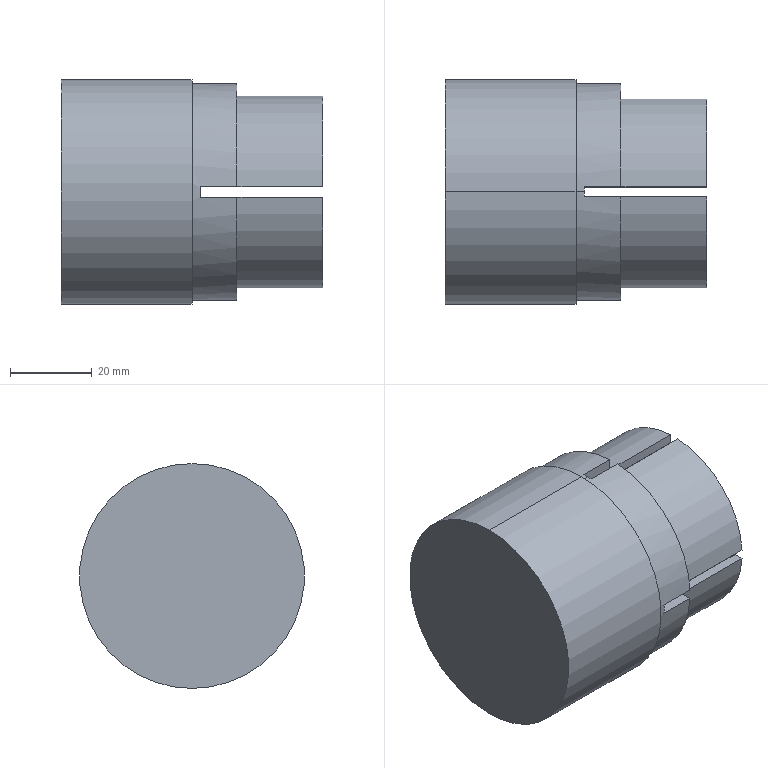Part | SolidWorks | features BaseBody 1 | 1 solid | 37 faces | box 64 x 55 x 55 mm | volume 51212 mm3 | plane 26 | cylinder 11 | commonest cylinder face diameters 47 x4 42.2 x3 53 x2 55 x2
STEP:
#1=CARTESIAN_POINT('',(34.,-1.25,-21.063));
#2=VERTEX_POINT('',#1);
#3=CARTESIAN_POINT('',(34.,0.,-21.1));
#4=VERTEX_POINT('',#3);
#5=CARTESIAN_POINT('',(34.,0.,0.));
#6=DIRECTION('',(1.,0.,0.));
#7=DIRECTION('',(0.,0.,1.));
#8=AXIS2_PLACEMENT_3D('',#5,#6,#7);
#9=CIRCLE('',#8,21.1);
#10=EDGE_CURVE('',#2,#4,#9,.T.);
#11=ORIENTED_EDGE('',*,*,#10,.T.);
#12=CARTESIAN_POINT('',(5.,0.,-21.1));
#13=VERTEX_POINT('',#12);
#14=CARTESIAN_POINT('',(-11.146,0.,-21.1));
#15=DIRECTION('',(-1.,0.,0.));
#16=VECTOR('',#15,1000.);
#17=LINE('',#14,#16);
#18=EDGE_CURVE('',#4,#13,#17,.T.);
#19=ORIENTED_EDGE('',*,*,#18,.T.);
#20=CARTESIAN_POINT('',(5.,0.,21.1));
#21=VERTEX_POINT('',#20);
#22=CARTESIAN_POINT('',(5.,0.,0.));
#23=DIRECTION('',(1.,0.,0.));
#24=DIRECTION('',(0.,0.,1.));
#25=AXIS2_PLACEMENT_3D('',#22,#23,#24);
#26=CIRCLE('',#25,21.1);
#27=EDGE_CURVE('',#21,#13,#26,.T.);
#28=ORIENTED_EDGE('',*,*,#27,.F.);
#29=CARTESIAN_POINT('',(34.,0.,21.1));
#30=VERTEX_POINT('',#29);
#31=CARTESIAN_POINT('',(-11.146,0.,21.1));
#32=DIRECTION('',(-1.,0.,0.));
#33=VECTOR('',#32,1000.);
#34=LINE('',#31,#33);
#35=EDGE_CURVE('',#30,#21,#34,.T.);
#36=ORIENTED_EDGE('',*,*,#35,.F.);
#37=CARTESIAN_POINT('',(34.,-1.25,21.063));
#38=VERTEX_POINT('',#37);
#39=CARTESIAN_POINT('',(34.,0.,0.));
#40=DIRECTION('',(1.,0.,0.));
#41=DIRECTION('',(0.,0.,1.));
#42=AXIS2_PLACEMENT_3D('',#39,#40,#41);
#43=CIRCLE('',#42,21.1);
#44=EDGE_CURVE('',#30,#38,#43,.T.);
#45=ORIENTED_EDGE('',*,*,#44,.T.);
#46=CARTESIAN_POINT('',(64.,-1.25,21.063));
#47=VERTEX_POINT('',#46);
#48=CARTESIAN_POINT('',(-11.146,-1.25,21.063));
#49=DIRECTION('',(-1.,0.,0.));
#50=VECTOR('',#49,1000.);
#51=LINE('',#48,#50);
#52=EDGE_CURVE('',#47,#38,#51,.T.);
#53=ORIENTED_EDGE('',*,*,#52,.F.);
#54=CARTESIAN_POINT('',(64.,-21.063,1.25));
#55=VERTEX_POINT('',#54);
#56=CARTESIAN_POINT('',(64.,0.,0.));
#57=DIRECTION('',(-1.,0.,0.));
#58=DIRECTION('',(0.,0.,1.));
#59=AXIS2_PLACEMENT_3D('',#56,#57,#58);
#60=CIRCLE('',#59,21.1);
#61=EDGE_CURVE('',#55,#47,#60,.T.);
#62=ORIENTED_EDGE('',*,*,#61,.F.);
#63=CARTESIAN_POINT('',(34.,-21.063,1.25));
#64=VERTEX_POINT('',#63);
#65=CARTESIAN_POINT('',(-11.146,-21.063,1.25));
#66=DIRECTION('',(1.,0.,0.));
#67=VECTOR('',#66,1000.);
#68=LINE('',#65,#67);
#69=EDGE_CURVE('',#64,#55,#68,.T.);
#70=ORIENTED_EDGE('',*,*,#69,.F.);
#71=CARTESIAN_POINT('',(34.,-21.063,-1.25));
#72=VERTEX_POINT('',#71);
#73=CARTESIAN_POINT('',(34.,0.,0.));
#74=DIRECTION('',(-1.,0.,0.));
#75=DIRECTION('',(0.,0.,1.));
#76=AXIS2_PLACEMENT_3D('',#73,#74,#75);
#77=CIRCLE('',#76,21.1);
#78=EDGE_CURVE('',#72,#64,#77,.T.);
#79=ORIENTED_EDGE('',*,*,#78,.F.);
#80=CARTESIAN_POINT('',(64.,-21.063,-1.25));
#81=VERTEX_POINT('',#80);
#82=CARTESIAN_POINT('',(-11.146,-21.063,-1.25));
#83=DIRECTION('',(-1.,0.,0.));
#84=VECTOR('',#83,1000.);
#85=LINE('',#82,#84);
#86=EDGE_CURVE('',#81,#72,#85,.T.);
#87=ORIENTED_EDGE('',*,*,#86,.F.);
#88=CARTESIAN_POINT('',(64.,-1.25,-21.063));
#89=VERTEX_POINT('',#88);
#90=CARTESIAN_POINT('',(64.,0.,0.));
#91=DIRECTION('',(-1.,0.,0.));
#92=DIRECTION('',(0.,0.,1.));
#93=AXIS2_PLACEMENT_3D('',#90,#91,#92);
#94=CIRCLE('',#93,21.1);
#95=EDGE_CURVE('',#89,#81,#94,.T.);
#96=ORIENTED_EDGE('',*,*,#95,.F.);
#97=CARTESIAN_POINT('',(-11.146,-1.25,-21.063));
#98=DIRECTION('',(1.,0.,0.));
#99=VECTOR('',#98,1000.);
#100=LINE('',#97,#99);
#101=EDGE_CURVE('',#2,#89,#100,.T.);
#102=ORIENTED_EDGE('',*,*,#101,.F.);
#103=EDGE_LOOP('',(#11,#19,#28,#36,#45,#53,#62,#70,#79,#87,#96,#102));
#104=FACE_OUTER_BOUND('',#103,.T.);
#105=CARTESIAN_POINT('',(-11.146,0.,0.));
#106=DIRECTION('',(-1.,0.,0.));
#107=DIRECTION('',(0.,0.,1.));
#108=AXIS2_PLACEMENT_3D('',#105,#106,#107);
#109=CYLINDRICAL_SURFACE('',#108,21.1);
#110=ADVANCED_FACE('',(#104),#109,.F.);
#111=CARTESIAN_POINT('',(34.,1.25,21.063));
#112=VERTEX_POINT('',#111);
#113=CARTESIAN_POINT('',(34.,0.,0.));
#114=DIRECTION('',(1.,0.,0.));
#115=DIRECTION('',(0.,0.,1.));
#116=AXIS2_PLACEMENT_3D('',#113,#114,#115);
#117=CIRCLE('',#116,21.1);
#118=EDGE_CURVE('',#112,#30,#117,.T.);
#119=ORIENTED_EDGE('',*,*,#118,.T.);
#120=ORIENTED_EDGE('',*,*,#35,.T.);
#121=CARTESIAN_POINT('',(5.,20.229,6.));
#122=VERTEX_POINT('',#121);
#123=CARTESIAN_POINT('',(5.,0.,0.));
#124=DIRECTION('',(1.,0.,0.));
#125=DIRECTION('',(0.,0.,1.));
#126=AXIS2_PLACEMENT_3D('',#123,#124,#125);
#127=CIRCLE('',#126,21.1);
#128=EDGE_CURVE('',#122,#21,#127,.T.);
#129=ORIENTED_EDGE('',*,*,#128,.F.);
#130=CARTESIAN_POINT('',(64.,20.229,6.));
#131=VERTEX_POINT('',#130);
#132=CARTESIAN_POINT('',(-11.146,20.229,6.));
#133=DIRECTION('',(-1.,0.,0.));
#134=VECTOR('',#133,1000.);
#135=LINE('',#132,#134);
#136=EDGE_CURVE('',#131,#122,#135,.T.);
#137=ORIENTED_EDGE('',*,*,#136,.F.);
#138=CARTESIAN_POINT('',(64.,1.25,21.063));
#139=VERTEX_POINT('',#138);
#140=CARTESIAN_POINT('',(64.,0.,0.));
#141=DIRECTION('',(-1.,0.,0.));
#142=DIRECTION('',(0.,0.,1.));
#143=AXIS2_PLACEMENT_3D('',#140,#141,#142);
#144=CIRCLE('',#143,21.1);
#145=EDGE_CURVE('',#139,#131,#144,.T.);
#146=ORIENTED_EDGE('',*,*,#145,.F.);
#147=CARTESIAN_POINT('',(-11.146,1.25,21.063));
#148=DIRECTION('',(1.,0.,0.));
#149=VECTOR('',#148,1000.);
#150=LINE('',#147,#149);
#151=EDGE_CURVE('',#112,#139,#150,.T.);
#152=ORIENTED_EDGE('',*,*,#151,.F.);
#153=EDGE_LOOP('',(#119,#120,#129,#137,#146,#152));
#154=FACE_OUTER_BOUND('',#153,.T.);
#155=CARTESIAN_POINT('',(-11.146,0.,0.));
#156=DIRECTION('',(-1.,0.,0.));
#157=DIRECTION('',(0.,0.,1.));
#158=AXIS2_PLACEMENT_3D('',#155,#156,#157);
#159=CYLINDRICAL_SURFACE('',#158,21.1);
#160=ADVANCED_FACE('',(#154),#159,.F.);
#161=CARTESIAN_POINT('',(34.,1.25,-26.471));
#162=VERTEX_POINT('',#161);
#163=CARTESIAN_POINT('',(34.,0.,-26.5));
#164=VERTEX_POINT('',#163);
#165=CARTESIAN_POINT('',(34.,0.,0.));
#166=DIRECTION('',(-1.,0.,0.));
#167=DIRECTION('',(0.,0.,1.));
#168=AXIS2_PLACEMENT_3D('',#165,#166,#167);
#169=CIRCLE('',#168,26.5);
#170=EDGE_CURVE('',#162,#164,#169,.T.);
#171=ORIENTED_EDGE('',*,*,#170,.T.);
#172=CARTESIAN_POINT('',(32.,0.,-26.5));
#173=VERTEX_POINT('',#172);
#174=CARTESIAN_POINT('',(-11.146,0.,-26.5));
#175=DIRECTION('',(-1.,0.,0.));
#176=VECTOR('',#175,1000.);
#177=LINE('',#174,#176);
#178=EDGE_CURVE('',#164,#173,#177,.T.);
#179=ORIENTED_EDGE('',*,*,#178,.T.);
#180=CARTESIAN_POINT('',(32.,0.,26.5));
#181=VERTEX_POINT('',#180);
#182=CARTESIAN_POINT('',(32.,0.,0.));
#183=DIRECTION('',(1.,0.,0.));
#184=DIRECTION('',(0.,0.,1.));
#185=AXIS2_PLACEMENT_3D('',#182,#183,#184);
#186=CIRCLE('',#185,26.5);
#187=EDGE_CURVE('',#173,#181,#186,.T.);
#188=ORIENTED_EDGE('',*,*,#187,.T.);
#189=CARTESIAN_POINT('',(34.,0.,26.5));
#190=VERTEX_POINT('',#189);
#191=CARTESIAN_POINT('',(-11.146,0.,26.5));
#192=DIRECTION('',(-1.,0.,0.));
#193=VECTOR('',#192,1000.);
#194=LINE('',#191,#193);
#195=EDGE_CURVE('',#190,#181,#194,.T.);
#196=ORIENTED_EDGE('',*,*,#195,.F.);
#197=CARTESIAN_POINT('',(34.,1.25,26.471));
#198=VERTEX_POINT('',#197);
#199=CARTESIAN_POINT('',(34.,0.,0.));
#200=DIRECTION('',(-1.,0.,0.));
#201=DIRECTION('',(0.,0.,1.));
#202=AXIS2_PLACEMENT_3D('',#199,#200,#201);
#203=CIRCLE('',#202,26.5);
#204=EDGE_CURVE('',#190,#198,#203,.T.);
#205=ORIENTED_EDGE('',*,*,#204,.T.);
#206=CARTESIAN_POINT('',(43.,1.25,26.471));
#207=VERTEX_POINT('',#206);
#208=CARTESIAN_POINT('',(34.,1.25,26.471));
#209=DIRECTION('',(1.,0.,0.));
#210=VECTOR('',#209,1000.);
#211=LINE('',#208,#210);
#212=EDGE_CURVE('',#198,#207,#211,.T.);
#213=ORIENTED_EDGE('',*,*,#212,.T.);
#214=CARTESIAN_POINT('',(43.,26.471,1.25));
#215=VERTEX_POINT('',#214);
#216=CARTESIAN_POINT('',(43.,0.,0.));
#217=DIRECTION('',(-1.,0.,0.));
#218=DIRECTION('',(0.,0.,1.));
#219=AXIS2_PLACEMENT_3D('',#216,#217,#218);
#220=CIRCLE('',#219,26.5);
#221=EDGE_CURVE('',#207,#215,#220,.T.);
#222=ORIENTED_EDGE('',*,*,#221,.T.);
#223=CARTESIAN_POINT('',(34.,26.471,1.25));
#224=VERTEX_POINT('',#223);
#225=CARTESIAN_POINT('',(-11.146,26.471,1.25));
#226=DIRECTION('',(-1.,0.,0.));
#227=VECTOR('',#226,1000.);
#228=LINE('',#225,#227);
#229=EDGE_CURVE('',#215,#224,#228,.T.);
#230=ORIENTED_EDGE('',*,*,#229,.T.);
#231=CARTESIAN_POINT('',(34.,26.471,-1.25));
#232=VERTEX_POINT('',#231);
#233=CARTESIAN_POINT('',(34.,0.,0.));
#234=DIRECTION('',(-1.,0.,0.));
#235=DIRECTION('',(0.,0.,1.));
#236=AXIS2_PLACEMENT_3D('',#233,#234,#235);
#237=CIRCLE('',#236,26.5);
#238=EDGE_CURVE('',#224,#232,#237,.T.);
#239=ORIENTED_EDGE('',*,*,#238,.T.);
#240=CARTESIAN_POINT('',(43.,26.471,-1.25));
#241=VERTEX_POINT('',#240);
#242=CARTESIAN_POINT('',(-11.146,26.471,-1.25));
#243=DIRECTION('',(1.,0.,0.));
#244=VECTOR('',#243,1000.);
#245=LINE('',#242,#244);
#246=EDGE_CURVE('',#232,#241,#245,.T.);
#247=ORIENTED_EDGE('',*,*,#246,.T.);
#248=CARTESIAN_POINT('',(43.,1.25,-26.471));
#249=VERTEX_POINT('',#248);
#250=CARTESIAN_POINT('',(43.,0.,0.));
#251=DIRECTION('',(-1.,0.,0.));
#252=DIRECTION('',(0.,0.,1.));
#253=AXIS2_PLACEMENT_3D('',#250,#251,#252);
#254=CIRCLE('',#253,26.5);
#255=EDGE_CURVE('',#241,#249,#254,.T.);
#256=ORIENTED_EDGE('',*,*,#255,.T.);
#257=CARTESIAN_POINT('',(34.,1.25,-26.471));
#258=DIRECTION('',(-1.,0.,0.));
#259=VECTOR('',#258,1000.);
#260=LINE('',#257,#259);
#261=EDGE_CURVE('',#249,#162,#260,.T.);
#262=ORIENTED_EDGE('',*,*,#261,.T.);
#263=EDGE_LOOP('',(#171,#179,#188,#196,#205,#213,#222,#230,#239,#247,#256,#262));
#264=FACE_OUTER_BOUND('',#263,.T.);
#265=CARTESIAN_POINT('',(-11.146,0.,0.));
#266=DIRECTION('',(-1.,0.,0.));
#267=DIRECTION('',(0.,0.,1.));
#268=AXIS2_PLACEMENT_3D('',#265,#266,#267);
#269=CYLINDRICAL_SURFACE('',#268,26.5);
#270=ADVANCED_FACE('',(#264),#269,.T.);
#271=CARTESIAN_POINT('',(32.,0.,27.5));
#272=VERTEX_POINT('',#271);
#273=CARTESIAN_POINT('',(32.,0.,-27.5));
#274=VERTEX_POINT('',#273);
#275=CARTESIAN_POINT('',(32.,0.,0.));
#276=DIRECTION('',(-1.,0.,0.));
#277=DIRECTION('',(0.,0.,1.));
#278=AXIS2_PLACEMENT_3D('',#275,#276,#277);
#279=CIRCLE('',#278,27.5);
#280=EDGE_CURVE('',#272,#274,#279,.T.);
#281=ORIENTED_EDGE('',*,*,#280,.T.);
#282=CARTESIAN_POINT('',(0.,0.,-27.5));
#283=VERTEX_POINT('',#282);
#284=CARTESIAN_POINT('',(-11.146,0.,-27.5));
#285=DIRECTION('',(-1.,0.,0.));
#286=VECTOR('',#285,1000.);
#287=LINE('',#284,#286);
#288=EDGE_CURVE('',#274,#283,#287,.T.);
#289=ORIENTED_EDGE('',*,*,#288,.T.);
#290=CARTESIAN_POINT('',(0.,0.,27.5));
#291=VERTEX_POINT('',#290);
#292=CARTESIAN_POINT('',(0.,0.,0.));
#293=DIRECTION('',(1.,0.,0.));
#294=DIRECTION('',(0.,0.,1.));
#295=AXIS2_PLACEMENT_3D('',#292,#293,#294);
#296=CIRCLE('',#295,27.5);
#297=EDGE_CURVE('',#283,#291,#296,.T.);
#298=ORIENTED_EDGE('',*,*,#297,.T.);
#299=CARTESIAN_POINT('',(-11.146,0.,27.5));
#300=DIRECTION('',(-1.,0.,0.));
#301=VECTOR('',#300,1000.);
#302=LINE('',#299,#301);
#303=EDGE_CURVE('',#272,#291,#302,.T.);
#304=ORIENTED_EDGE('',*,*,#303,.F.);
#305=EDGE_LOOP('',(#281,#289,#298,#304));
#306=FACE_OUTER_BOUND('',#305,.T.);
#307=CARTESIAN_POINT('',(-11.146,0.,0.));
#308=DIRECTION('',(-1.,0.,0.));
#309=DIRECTION('',(0.,0.,1.));
#310=AXIS2_PLACEMENT_3D('',#307,#308,#309);
#311=CYLINDRICAL_SURFACE('',#310,27.5);
#312=ADVANCED_FACE('',(#306),#311,.T.);
#313=ORIENTED_EDGE('',*,*,#18,.F.);
#314=CARTESIAN_POINT('',(34.,1.25,-21.063));
#315=VERTEX_POINT('',#314);
#316=CARTESIAN_POINT('',(34.,0.,0.));
#317=DIRECTION('',(1.,0.,0.));
#318=DIRECTION('',(0.,0.,1.));
#319=AXIS2_PLACEMENT_3D('',#316,#317,#318);
#320=CIRCLE('',#319,21.1);
#321=EDGE_CURVE('',#4,#315,#320,.T.);
#322=ORIENTED_EDGE('',*,*,#321,.T.);
#323=CARTESIAN_POINT('',(64.,1.25,-21.063));
#324=VERTEX_POINT('',#323);
#325=CARTESIAN_POINT('',(-11.146,1.25,-21.063));
#326=DIRECTION('',(-1.,0.,0.));
#327=VECTOR('',#326,1000.);
#328=LINE('',#325,#327);
#329=EDGE_CURVE('',#324,#315,#328,.T.);
#330=ORIENTED_EDGE('',*,*,#329,.F.);
#331=CARTESIAN_POINT('',(64.,20.229,-6.));
#332=VERTEX_POINT('',#331);
#333=CARTESIAN_POINT('',(64.,0.,0.));
#334=DIRECTION('',(-1.,0.,0.));
#335=DIRECTION('',(0.,0.,1.));
#336=AXIS2_PLACEMENT_3D('',#333,#334,#335);
#337=CIRCLE('',#336,21.1);
#338=EDGE_CURVE('',#332,#324,#337,.T.);
#339=ORIENTED_EDGE('',*,*,#338,.F.);
#340=CARTESIAN_POINT('',(5.,20.229,-6.));
#341=VERTEX_POINT('',#340);
#342=CARTESIAN_POINT('',(-11.146,20.229,-6.));
#343=DIRECTION('',(1.,0.,0.));
#344=VECTOR('',#343,1000.);
#345=LINE('',#342,#344);
#346=EDGE_CURVE('',#341,#332,#345,.T.);
#347=ORIENTED_EDGE('',*,*,#346,.F.);
#348=CARTESIAN_POINT('',(5.,0.,0.));
#349=DIRECTION('',(1.,0.,0.));
#350=DIRECTION('',(0.,0.,1.));
#351=AXIS2_PLACEMENT_3D('',#348,#349,#350);
#352=CIRCLE('',#351,21.1);
#353=EDGE_CURVE('',#13,#341,#352,.T.);
#354=ORIENTED_EDGE('',*,*,#353,.F.);
#355=EDGE_LOOP('',(#313,#322,#330,#339,#347,#354));
#356=FACE_OUTER_BOUND('',#355,.T.);
#357=CARTESIAN_POINT('',(-11.146,0.,0.));
#358=DIRECTION('',(-1.,0.,0.));
#359=DIRECTION('',(0.,0.,1.));
#360=AXIS2_PLACEMENT_3D('',#357,#358,#359);
#361=CYLINDRICAL_SURFACE('',#360,21.1);
#362=ADVANCED_FACE('',(#356),#361,.F.);
#363=CARTESIAN_POINT('',(5.,24.3,6.));
#364=VERTEX_POINT('',#363);
#365=CARTESIAN_POINT('',(5.,24.3,-6.));
#366=VERTEX_POINT('',#365);
#367=CARTESIAN_POINT('',(5.,24.3,0.));
#368=DIRECTION('',(0.,0.,-1.));
#369=VECTOR('',#368,1000.);
#370=LINE('',#367,#369);
#371=EDGE_CURVE('',#364,#366,#370,.T.);
#372=ORIENTED_EDGE('',*,*,#371,.F.);
#373=CARTESIAN_POINT('',(5.,21.1,6.));
#374=DIRECTION('',(0.,1.,0.));
#375=VECTOR('',#374,1000.);
#376=LINE('',#373,#375);
#377=EDGE_CURVE('',#122,#364,#376,.T.);
#378=ORIENTED_EDGE('',*,*,#377,.F.);
#379=ORIENTED_EDGE('',*,*,#128,.T.);
#380=ORIENTED_EDGE('',*,*,#27,.T.);
#381=ORIENTED_EDGE('',*,*,#353,.T.);
#382=CARTESIAN_POINT('',(5.,21.1,-6.));
#383=DIRECTION('',(0.,-1.,0.));
#384=VECTOR('',#383,1000.);
#385=LINE('',#382,#384);
#386=EDGE_CURVE('',#366,#341,#385,.T.);
#387=ORIENTED_EDGE('',*,*,#386,.F.);
#388=EDGE_LOOP('',(#372,#378,#379,#380,#381,#387));
#389=FACE_OUTER_BOUND('',#388,.T.);
#390=CARTESIAN_POINT('',(5.,21.1,0.));
#391=DIRECTION('',(-1.,0.,0.));
#392=DIRECTION('',(0.,0.,1.));
#393=AXIS2_PLACEMENT_3D('',#390,#391,#392);
#394=PLANE('',#393);
#395=ADVANCED_FACE('',(#389),#394,.F.);
#396=CARTESIAN_POINT('',(34.,-1.25,26.471));
#397=VERTEX_POINT('',#396);
#398=CARTESIAN_POINT('',(34.,-1.25,33.123));
#399=DIRECTION('',(0.,0.,-1.));
#400=VECTOR('',#399,1000.);
#401=LINE('',#398,#400);
#402=EDGE_CURVE('',#397,#38,#401,.T.);
#403=ORIENTED_EDGE('',*,*,#402,.F.);
#404=CARTESIAN_POINT('',(43.,-1.25,26.471));
#405=VERTEX_POINT('',#404);
#406=CARTESIAN_POINT('',(34.,-1.25,26.471));
#407=DIRECTION('',(-1.,0.,0.));
#408=VECTOR('',#407,1000.);
#409=LINE('',#406,#408);
#410=EDGE_CURVE('',#405,#397,#409,.T.);
#411=ORIENTED_EDGE('',*,*,#410,.F.);
#412=CARTESIAN_POINT('',(43.,-1.25,23.467));
#413=VERTEX_POINT('',#412);
#414=CARTESIAN_POINT('',(43.,-1.25,33.123));
#415=DIRECTION('',(0.,0.,1.));
#416=VECTOR('',#415,1000.);
#417=LINE('',#414,#416);
#418=EDGE_CURVE('',#413,#405,#417,.T.);
#419=ORIENTED_EDGE('',*,*,#418,.F.);
#420=CARTESIAN_POINT('',(64.,-1.25,23.467));
#421=VERTEX_POINT('',#420);
#422=CARTESIAN_POINT('',(34.,-1.25,23.467));
#423=DIRECTION('',(-1.,0.,0.));
#424=VECTOR('',#423,1000.);
#425=LINE('',#422,#424);
#426=EDGE_CURVE('',#421,#413,#425,.T.);
#427=ORIENTED_EDGE('',*,*,#426,.F.);
#428=CARTESIAN_POINT('',(64.,-1.25,33.123));
#429=DIRECTION('',(0.,0.,1.));
#430=VECTOR('',#429,1000.);
#431=LINE('',#428,#430);
#432=EDGE_CURVE('',#47,#421,#431,.T.);
#433=ORIENTED_EDGE('',*,*,#432,.F.);
#434=ORIENTED_EDGE('',*,*,#52,.T.);
#435=EDGE_LOOP('',(#403,#411,#419,#427,#433,#434));
#436=FACE_OUTER_BOUND('',#435,.T.);
#437=CARTESIAN_POINT('',(34.,-1.25,33.123));
#438=DIRECTION('',(0.,-1.,0.));
#439=DIRECTION('',(0.,0.,-1.));
#440=AXIS2_PLACEMENT_3D('',#437,#438,#439);
#441=PLANE('',#440);
#442=ADVANCED_FACE('',(#436),#441,.F.);
#443=ORIENTED_EDGE('',*,*,#432,.T.);
#444=CARTESIAN_POINT('',(64.,-23.467,1.25));
#445=VERTEX_POINT('',#444);
#446=CARTESIAN_POINT('',(64.,0.,0.));
#447=DIRECTION('',(-1.,0.,0.));
#448=DIRECTION('',(0.,0.,1.));
#449=AXIS2_PLACEMENT_3D('',#446,#447,#448);
#450=CIRCLE('',#449,23.5);
#451=EDGE_CURVE('',#445,#421,#450,.T.);
#452=ORIENTED_EDGE('',*,*,#451,.F.);
#453=CARTESIAN_POINT('',(64.,23.5,1.25));
#454=DIRECTION('',(0.,-1.,0.));
#455=VECTOR('',#454,1000.);
#456=LINE('',#453,#455);
#457=EDGE_CURVE('',#55,#445,#456,.T.);
#458=ORIENTED_EDGE('',*,*,#457,.F.);
#459=ORIENTED_EDGE('',*,*,#61,.T.);
#460=EDGE_LOOP('',(#443,#452,#458,#459));
#461=FACE_OUTER_BOUND('',#460,.T.);
#462=CARTESIAN_POINT('',(64.,23.5,0.));
#463=DIRECTION('',(-1.,0.,0.));
#464=DIRECTION('',(0.,0.,1.));
#465=AXIS2_PLACEMENT_3D('',#462,#463,#464);
#466=PLANE('',#465);
#467=ADVANCED_FACE('',(#461),#466,.F.);
#468=CARTESIAN_POINT('',(43.,-23.467,1.25));
#469=VERTEX_POINT('',#468);
#470=CARTESIAN_POINT('',(34.,-23.467,1.25));
#471=DIRECTION('',(1.,0.,0.));
#472=VECTOR('',#471,1000.);
#473=LINE('',#470,#472);
#474=EDGE_CURVE('',#469,#445,#473,.T.);
#475=ORIENTED_EDGE('',*,*,#474,.F.);
#476=CARTESIAN_POINT('',(43.,-26.471,1.25));
#477=VERTEX_POINT('',#476);
#478=CARTESIAN_POINT('',(43.,-33.123,1.25));
#479=DIRECTION('',(0.,1.,0.));
#480=VECTOR('',#479,1000.);
#481=LINE('',#478,#480);
#482=EDGE_CURVE('',#477,#469,#481,.T.);
#483=ORIENTED_EDGE('',*,*,#482,.F.);
#484=CARTESIAN_POINT('',(34.,-26.471,1.25));
#485=VERTEX_POINT('',#484);
#486=CARTESIAN_POINT('',(34.,-26.471,1.25));
#487=DIRECTION('',(1.,0.,0.));
#488=VECTOR('',#487,1000.);
#489=LINE('',#486,#488);
#490=EDGE_CURVE('',#485,#477,#489,.T.);
#491=ORIENTED_EDGE('',*,*,#490,.F.);
#492=CARTESIAN_POINT('',(34.,-33.123,1.25));
#493=DIRECTION('',(0.,-1.,0.));
#494=VECTOR('',#493,1000.);
#495=LINE('',#492,#494);
#496=EDGE_CURVE('',#64,#485,#495,.T.);
#497=ORIENTED_EDGE('',*,*,#496,.F.);
#498=ORIENTED_EDGE('',*,*,#69,.T.);
#499=ORIENTED_EDGE('',*,*,#457,.T.);
#500=EDGE_LOOP('',(#475,#483,#491,#497,#498,#499));
#501=FACE_OUTER_BOUND('',#500,.T.);
#502=CARTESIAN_POINT('',(34.,-33.123,1.25));
#503=DIRECTION('',(0.,0.,1.));
#504=DIRECTION('',(1.,0.,0.));
#505=AXIS2_PLACEMENT_3D('',#502,#503,#504);
#506=PLANE('',#505);
#507=ADVANCED_FACE('',(#501),#506,.F.);
#508=CARTESIAN_POINT('',(34.,-26.471,-1.25));
#509=VERTEX_POINT('',#508);
#510=CARTESIAN_POINT('',(34.,33.123,-1.25));
#511=DIRECTION('',(0.,-1.,0.));
#512=VECTOR('',#511,1000.);
#513=LINE('',#510,#512);
#514=EDGE_CURVE('',#72,#509,#513,.T.);
#515=ORIENTED_EDGE('',*,*,#514,.F.);
#516=ORIENTED_EDGE('',*,*,#78,.T.);
#517=ORIENTED_EDGE('',*,*,#496,.T.);
#518=CARTESIAN_POINT('',(34.,0.,0.));
#519=DIRECTION('',(-1.,0.,0.));
#520=DIRECTION('',(0.,0.,1.));
#521=AXIS2_PLACEMENT_3D('',#518,#519,#520);
#522=CIRCLE('',#521,26.5);
#523=EDGE_CURVE('',#509,#485,#522,.T.);
#524=ORIENTED_EDGE('',*,*,#523,.F.);
#525=EDGE_LOOP('',(#515,#516,#517,#524));
#526=FACE_OUTER_BOUND('',#525,.T.);
#527=CARTESIAN_POINT('',(34.,33.123,-1.25));
#528=DIRECTION('',(-1.,0.,0.));
#529=DIRECTION('',(0.,0.,1.));
#530=AXIS2_PLACEMENT_3D('',#527,#528,#529);
#531=PLANE('',#530);
#532=ADVANCED_FACE('',(#526),#531,.F.);
#533=ORIENTED_EDGE('',*,*,#514,.T.);
#534=CARTESIAN_POINT('',(43.,-26.471,-1.25));
#535=VERTEX_POINT('',#534);
#536=CARTESIAN_POINT('',(34.,-26.471,-1.25));
#537=DIRECTION('',(-1.,0.,0.));
#538=VECTOR('',#537,1000.);
#539=LINE('',#536,#538);
#540=EDGE_CURVE('',#535,#509,#539,.T.);
#541=ORIENTED_EDGE('',*,*,#540,.F.);
#542=CARTESIAN_POINT('',(43.,-23.467,-1.25));
#543=VERTEX_POINT('',#542);
#544=CARTESIAN_POINT('',(43.,-33.123,-1.25));
#545=DIRECTION('',(0.,-1.,0.));
#546=VECTOR('',#545,1000.);
#547=LINE('',#544,#546);
#548=EDGE_CURVE('',#543,#535,#547,.T.);
#549=ORIENTED_EDGE('',*,*,#548,.F.);
#550=CARTESIAN_POINT('',(64.,-23.467,-1.25));
#551=VERTEX_POINT('',#550);
#552=CARTESIAN_POINT('',(34.,-23.467,-1.25));
#553=DIRECTION('',(-1.,0.,0.));
#554=VECTOR('',#553,1000.);
#555=LINE('',#552,#554);
#556=EDGE_CURVE('',#551,#543,#555,.T.);
#557=ORIENTED_EDGE('',*,*,#556,.F.);
#558=CARTESIAN_POINT('',(64.,-33.123,-1.25));
#559=DIRECTION('',(0.,-1.,0.));
#560=VECTOR('',#559,1000.);
#561=LINE('',#558,#560);
#562=EDGE_CURVE('',#81,#551,#561,.T.);
#563=ORIENTED_EDGE('',*,*,#562,.F.);
#564=ORIENTED_EDGE('',*,*,#86,.T.);
#565=EDGE_LOOP('',(#533,#541,#549,#557,#563,#564));
#566=FACE_OUTER_BOUND('',#565,.T.);
#567=CARTESIAN_POINT('',(34.,-33.123,-1.25));
#568=DIRECTION('',(0.,0.,-1.));
#569=DIRECTION('',(-1.,0.,0.));
#570=AXIS2_PLACEMENT_3D('',#567,#568,#569);
#571=PLANE('',#570);
#572=ADVANCED_FACE('',(#566),#571,.F.);
#573=ORIENTED_EDGE('',*,*,#562,.T.);
#574=CARTESIAN_POINT('',(64.,-1.25,-23.467));
#575=VERTEX_POINT('',#574);
#576=CARTESIAN_POINT('',(64.,0.,0.));
#577=DIRECTION('',(-1.,0.,0.));
#578=DIRECTION('',(0.,0.,1.));
#579=AXIS2_PLACEMENT_3D('',#576,#577,#578);
#580=CIRCLE('',#579,23.5);
#581=EDGE_CURVE('',#575,#551,#580,.T.);
#582=ORIENTED_EDGE('',*,*,#581,.F.);
#583=CARTESIAN_POINT('',(64.,-1.25,0.));
#584=DIRECTION('',(0.,0.,-1.));
#585=VECTOR('',#584,1000.);
#586=LINE('',#583,#585);
#587=EDGE_CURVE('',#89,#575,#586,.T.);
#588=ORIENTED_EDGE('',*,*,#587,.F.);
#589=ORIENTED_EDGE('',*,*,#95,.T.);
#590=EDGE_LOOP('',(#573,#582,#588,#589));
#591=FACE_OUTER_BOUND('',#590,.T.);
#592=CARTESIAN_POINT('',(64.,23.5,0.));
#593=DIRECTION('',(-1.,0.,0.));
#594=DIRECTION('',(0.,0.,1.));
#595=AXIS2_PLACEMENT_3D('',#592,#593,#594);
#596=PLANE('',#595);
#597=ADVANCED_FACE('',(#591),#596,.F.);
#598=CARTESIAN_POINT('',(43.,-1.25,-23.467));
#599=VERTEX_POINT('',#598);
#600=CARTESIAN_POINT('',(34.,-1.25,-23.467));
#601=DIRECTION('',(1.,0.,0.));
#602=VECTOR('',#601,1000.);
#603=LINE('',#600,#602);
#604=EDGE_CURVE('',#599,#575,#603,.T.);
#605=ORIENTED_EDGE('',*,*,#604,.F.);
#606=CARTESIAN_POINT('',(43.,-1.25,-26.471));
#607=VERTEX_POINT('',#606);
#608=CARTESIAN_POINT('',(43.,-1.25,33.123));
#609=DIRECTION('',(0.,0.,1.));
#610=VECTOR('',#609,1000.);
#611=LINE('',#608,#610);
#612=EDGE_CURVE('',#607,#599,#611,.T.);
#613=ORIENTED_EDGE('',*,*,#612,.F.);
#614=CARTESIAN_POINT('',(34.,-1.25,-26.471));
#615=VERTEX_POINT('',#614);
#616=CARTESIAN_POINT('',(34.,-1.25,-26.471));
#617=DIRECTION('',(1.,0.,0.));
#618=VECTOR('',#617,1000.);
#619=LINE('',#616,#618);
#620=EDGE_CURVE('',#615,#607,#619,.T.);
#621=ORIENTED_EDGE('',*,*,#620,.F.);
#622=CARTESIAN_POINT('',(34.,-1.25,33.123));
#623=DIRECTION('',(0.,0.,-1.));
#624=VECTOR('',#623,1000.);
#625=LINE('',#622,#624);
#626=EDGE_CURVE('',#2,#615,#625,.T.);
#627=ORIENTED_EDGE('',*,*,#626,.F.);
#628=ORIENTED_EDGE('',*,*,#101,.T.);
#629=ORIENTED_EDGE('',*,*,#587,.T.);
#630=EDGE_LOOP('',(#605,#613,#621,#627,#628,#629));
#631=FACE_OUTER_BOUND('',#630,.T.);
#632=CARTESIAN_POINT('',(34.,-1.25,33.123));
#633=DIRECTION('',(0.,-1.,0.));
#634=DIRECTION('',(0.,0.,-1.));
#635=AXIS2_PLACEMENT_3D('',#632,#633,#634);
#636=PLANE('',#635);
#637=ADVANCED_FACE('',(#631),#636,.F.);
#638=CARTESIAN_POINT('',(34.,1.25,33.123));
#639=DIRECTION('',(0.,0.,1.));
#640=VECTOR('',#639,1000.);
#641=LINE('',#638,#640);
#642=EDGE_CURVE('',#162,#315,#641,.T.);
#643=ORIENTED_EDGE('',*,*,#642,.F.);
#644=ORIENTED_EDGE('',*,*,#261,.F.);
#645=CARTESIAN_POINT('',(43.,1.25,-23.467));
#646=VERTEX_POINT('',#645);
#647=CARTESIAN_POINT('',(43.,1.25,33.123));
#648=DIRECTION('',(0.,0.,-1.));
#649=VECTOR('',#648,1000.);
#650=LINE('',#647,#649);
#651=EDGE_CURVE('',#646,#249,#650,.T.);
#652=ORIENTED_EDGE('',*,*,#651,.F.);
#653=CARTESIAN_POINT('',(64.,1.25,-23.467));
#654=VERTEX_POINT('',#653);
#655=CARTESIAN_POINT('',(34.,1.25,-23.467));
#656=DIRECTION('',(-1.,0.,0.));
#657=VECTOR('',#656,1000.);
#658=LINE('',#655,#657);
#659=EDGE_CURVE('',#654,#646,#658,.T.);
#660=ORIENTED_EDGE('',*,*,#659,.F.);
#661=CARTESIAN_POINT('',(64.,1.25,33.123));
#662=DIRECTION('',(0.,0.,-1.));
#663=VECTOR('',#662,1000.);
#664=LINE('',#661,#663);
#665=EDGE_CURVE('',#324,#654,#664,.T.);
#666=ORIENTED_EDGE('',*,*,#665,.F.);
#667=ORIENTED_EDGE('',*,*,#329,.T.);
#668=EDGE_LOOP('',(#643,#644,#652,#660,#666,#667));
#669=FACE_OUTER_BOUND('',#668,.T.);
#670=CARTESIAN_POINT('',(34.,1.25,33.123));
#671=DIRECTION('',(0.,1.,0.));
#672=DIRECTION('',(0.,0.,1.));
#673=AXIS2_PLACEMENT_3D('',#670,#671,#672);
#674=PLANE('',#673);
#675=ADVANCED_FACE('',(#669),#674,.F.);
#676=ORIENTED_EDGE('',*,*,#665,.T.);
#677=CARTESIAN_POINT('',(64.,22.721,-6.));
#678=VERTEX_POINT('',#677);
#679=CARTESIAN_POINT('',(64.,0.,0.));
#680=DIRECTION('',(-1.,0.,0.));
#681=DIRECTION('',(0.,0.,1.));
#682=AXIS2_PLACEMENT_3D('',#679,#680,#681);
#683=CIRCLE('',#682,23.5);
#684=EDGE_CURVE('',#678,#654,#683,.T.);
#685=ORIENTED_EDGE('',*,*,#684,.F.);
#686=CARTESIAN_POINT('',(64.,23.5,-6.));
#687=DIRECTION('',(0.,1.,0.));
#688=VECTOR('',#687,1000.);
#689=LINE('',#686,#688);
#690=EDGE_CURVE('',#332,#678,#689,.T.);
#691=ORIENTED_EDGE('',*,*,#690,.F.);
#692=ORIENTED_EDGE('',*,*,#338,.T.);
#693=EDGE_LOOP('',(#676,#685,#691,#692));
#694=FACE_OUTER_BOUND('',#693,.T.);
#695=CARTESIAN_POINT('',(64.,23.5,0.));
#696=DIRECTION('',(-1.,0.,0.));
#697=DIRECTION('',(0.,0.,1.));
#698=AXIS2_PLACEMENT_3D('',#695,#696,#697);
#699=PLANE('',#698);
#700=ADVANCED_FACE('',(#694),#699,.F.);
#701=CARTESIAN_POINT('',(43.,22.721,-6.));
#702=VERTEX_POINT('',#701);
#703=CARTESIAN_POINT('',(-16.436,22.721,-6.));
#704=DIRECTION('',(1.,0.,0.));
#705=VECTOR('',#704,1000.);
#706=LINE('',#703,#705);
#707=EDGE_CURVE('',#702,#678,#706,.T.);
#708=ORIENTED_EDGE('',*,*,#707,.F.);
#709=CARTESIAN_POINT('',(43.,24.3,-6.));
#710=VERTEX_POINT('',#709);
#711=CARTESIAN_POINT('',(43.,24.3,-6.));
#712=DIRECTION('',(0.,-1.,0.));
#713=VECTOR('',#712,1000.);
#714=LINE('',#711,#713);
#715=EDGE_CURVE('',#710,#702,#714,.T.);
#716=ORIENTED_EDGE('',*,*,#715,.F.);
#717=CARTESIAN_POINT('',(-16.436,24.3,-6.));
#718=DIRECTION('',(1.,0.,0.));
#719=VECTOR('',#718,1000.);
#720=LINE('',#717,#719);
#721=EDGE_CURVE('',#366,#710,#720,.T.);
#722=ORIENTED_EDGE('',*,*,#721,.F.);
#723=ORIENTED_EDGE('',*,*,#386,.T.);
#724=ORIENTED_EDGE('',*,*,#346,.T.);
#725=ORIENTED_EDGE('',*,*,#690,.T.);
#726=EDGE_LOOP('',(#708,#716,#722,#723,#724,#725));
#727=FACE_OUTER_BOUND('',#726,.T.);
#728=CARTESIAN_POINT('',(-16.436,24.3,-6.));
#729=DIRECTION('',(0.,0.,-1.));
#730=DIRECTION('',(-1.,0.,0.));
#731=AXIS2_PLACEMENT_3D('',#728,#729,#730);
#732=PLANE('',#731);
#733=ADVANCED_FACE('',(#727),#732,.F.);
#734=CARTESIAN_POINT('',(34.,24.3,1.25));
#735=VERTEX_POINT('',#734);
#736=CARTESIAN_POINT('',(34.,24.3,-1.25));
#737=VERTEX_POINT('',#736);
#738=CARTESIAN_POINT('',(34.,24.3,6.));
#739=DIRECTION('',(0.,0.,-1.));
#740=VECTOR('',#739,1000.);
#741=LINE('',#738,#740);
#742=EDGE_CURVE('',#735,#737,#741,.T.);
#743=ORIENTED_EDGE('',*,*,#742,.F.);
#744=CARTESIAN_POINT('',(43.,24.3,1.25));
#745=VERTEX_POINT('',#744);
#746=CARTESIAN_POINT('',(-16.436,24.3,1.25));
#747=DIRECTION('',(-1.,0.,0.));
#748=VECTOR('',#747,1000.);
#749=LINE('',#746,#748);
#750=EDGE_CURVE('',#745,#735,#749,.T.);
#751=ORIENTED_EDGE('',*,*,#750,.F.);
#752=CARTESIAN_POINT('',(43.,24.3,6.));
#753=VERTEX_POINT('',#752);
#754=CARTESIAN_POINT('',(43.,24.3,6.));
#755=DIRECTION('',(0.,0.,-1.));
#756=VECTOR('',#755,1000.);
#757=LINE('',#754,#756);
#758=EDGE_CURVE('',#753,#745,#757,.T.);
#759=ORIENTED_EDGE('',*,*,#758,.F.);
#760=CARTESIAN_POINT('',(-16.436,24.3,6.));
#761=DIRECTION('',(1.,0.,0.));
#762=VECTOR('',#761,1000.);
#763=LINE('',#760,#762);
#764=EDGE_CURVE('',#364,#753,#763,.T.);
#765=ORIENTED_EDGE('',*,*,#764,.F.);
#766=ORIENTED_EDGE('',*,*,#371,.T.);
#767=ORIENTED_EDGE('',*,*,#721,.T.);
#768=CARTESIAN_POINT('',(43.,24.3,-1.25));
#769=VERTEX_POINT('',#768);
#770=CARTESIAN_POINT('',(43.,24.3,6.));
#771=DIRECTION('',(0.,0.,-1.));
#772=VECTOR('',#771,1000.);
#773=LINE('',#770,#772);
#774=EDGE_CURVE('',#769,#710,#773,.T.);
#775=ORIENTED_EDGE('',*,*,#774,.F.);
#776=CARTESIAN_POINT('',(-16.436,24.3,-1.25));
#777=DIRECTION('',(1.,0.,0.));
#778=VECTOR('',#777,1000.);
#779=LINE('',#776,#778);
#780=EDGE_CURVE('',#737,#769,#779,.T.);
#781=ORIENTED_EDGE('',*,*,#780,.F.);
#782=EDGE_LOOP('',(#743,#751,#759,#765,#766,#767,#775,#781));
#783=FACE_OUTER_BOUND('',#782,.T.);
#784=CARTESIAN_POINT('',(-16.436,24.3,6.));
#785=DIRECTION('',(0.,1.,0.));
#786=DIRECTION('',(0.,0.,1.));
#787=AXIS2_PLACEMENT_3D('',#784,#785,#786);
#788=PLANE('',#787);
#789=ADVANCED_FACE('',(#783),#788,.F.);
#790=ORIENTED_EDGE('',*,*,#377,.T.);
#791=ORIENTED_EDGE('',*,*,#764,.T.);
#792=CARTESIAN_POINT('',(43.,22.721,6.));
#793=VERTEX_POINT('',#792);
#794=CARTESIAN_POINT('',(43.,24.3,6.));
#795=DIRECTION('',(0.,1.,0.));
#796=VECTOR('',#795,1000.);
#797=LINE('',#794,#796);
#798=EDGE_CURVE('',#793,#753,#797,.T.);
#799=ORIENTED_EDGE('',*,*,#798,.F.);
#800=CARTESIAN_POINT('',(64.,22.721,6.));
#801=VERTEX_POINT('',#800);
#802=CARTESIAN_POINT('',(-16.436,22.721,6.));
#803=DIRECTION('',(-1.,0.,0.));
#804=VECTOR('',#803,1000.);
#805=LINE('',#802,#804);
#806=EDGE_CURVE('',#801,#793,#805,.T.);
#807=ORIENTED_EDGE('',*,*,#806,.F.);
#808=CARTESIAN_POINT('',(64.,24.3,6.));
#809=DIRECTION('',(0.,1.,0.));
#810=VECTOR('',#809,1000.);
#811=LINE('',#808,#810);
#812=EDGE_CURVE('',#131,#801,#811,.T.);
#813=ORIENTED_EDGE('',*,*,#812,.F.);
#814=ORIENTED_EDGE('',*,*,#136,.T.);
#815=EDGE_LOOP('',(#790,#791,#799,#807,#813,#814));
#816=FACE_OUTER_BOUND('',#815,.T.);
#817=CARTESIAN_POINT('',(-16.436,24.3,6.));
#818=DIRECTION('',(0.,0.,1.));
#819=DIRECTION('',(1.,0.,0.));
#820=AXIS2_PLACEMENT_3D('',#817,#818,#819);
#821=PLANE('',#820);
#822=ADVANCED_FACE('',(#816),#821,.F.);
#823=ORIENTED_EDGE('',*,*,#812,.T.);
#824=CARTESIAN_POINT('',(64.,1.25,23.467));
#825=VERTEX_POINT('',#824);
#826=CARTESIAN_POINT('',(64.,0.,0.));
#827=DIRECTION('',(-1.,0.,0.));
#828=DIRECTION('',(0.,0.,1.));
#829=AXIS2_PLACEMENT_3D('',#826,#827,#828);
#830=CIRCLE('',#829,23.5);
#831=EDGE_CURVE('',#825,#801,#830,.T.);
#832=ORIENTED_EDGE('',*,*,#831,.F.);
#833=CARTESIAN_POINT('',(64.,1.25,0.));
#834=DIRECTION('',(0.,0.,1.));
#835=VECTOR('',#834,1000.);
#836=LINE('',#833,#835);
#837=EDGE_CURVE('',#139,#825,#836,.T.);
#838=ORIENTED_EDGE('',*,*,#837,.F.);
#839=ORIENTED_EDGE('',*,*,#145,.T.);
#840=EDGE_LOOP('',(#823,#832,#838,#839));
#841=FACE_OUTER_BOUND('',#840,.T.);
#842=CARTESIAN_POINT('',(64.,23.5,0.));
#843=DIRECTION('',(-1.,0.,0.));
#844=DIRECTION('',(0.,0.,1.));
#845=AXIS2_PLACEMENT_3D('',#842,#843,#844);
#846=PLANE('',#845);
#847=ADVANCED_FACE('',(#841),#846,.F.);
#848=CARTESIAN_POINT('',(43.,1.25,23.467));
#849=VERTEX_POINT('',#848);
#850=CARTESIAN_POINT('',(34.,1.25,23.467));
#851=DIRECTION('',(1.,0.,0.));
#852=VECTOR('',#851,1000.);
#853=LINE('',#850,#852);
#854=EDGE_CURVE('',#849,#825,#853,.T.);
#855=ORIENTED_EDGE('',*,*,#854,.F.);
#856=CARTESIAN_POINT('',(43.,1.25,33.123));
#857=DIRECTION('',(0.,0.,-1.));
#858=VECTOR('',#857,1000.);
#859=LINE('',#856,#858);
#860=EDGE_CURVE('',#207,#849,#859,.T.);
#861=ORIENTED_EDGE('',*,*,#860,.F.);
#862=ORIENTED_EDGE('',*,*,#212,.F.);
#863=CARTESIAN_POINT('',(34.,1.25,33.123));
#864=DIRECTION('',(0.,0.,1.));
#865=VECTOR('',#864,1000.);
#866=LINE('',#863,#865);
#867=EDGE_CURVE('',#112,#198,#866,.T.);
#868=ORIENTED_EDGE('',*,*,#867,.F.);
#869=ORIENTED_EDGE('',*,*,#151,.T.);
#870=ORIENTED_EDGE('',*,*,#837,.T.);
#871=EDGE_LOOP('',(#855,#861,#862,#868,#869,#870));
#872=FACE_OUTER_BOUND('',#871,.T.);
#873=CARTESIAN_POINT('',(34.,1.25,33.123));
#874=DIRECTION('',(0.,1.,0.));
#875=DIRECTION('',(0.,0.,1.));
#876=AXIS2_PLACEMENT_3D('',#873,#874,#875);
#877=PLANE('',#876);
#878=ADVANCED_FACE('',(#872),#877,.F.);
#879=CARTESIAN_POINT('',(34.,0.,0.));
#880=DIRECTION('',(-1.,0.,0.));
#881=DIRECTION('',(0.,0.,1.));
#882=AXIS2_PLACEMENT_3D('',#879,#880,#881);
#883=CIRCLE('',#882,26.5);
#884=EDGE_CURVE('',#397,#190,#883,.T.);
#885=ORIENTED_EDGE('',*,*,#884,.F.);
#886=ORIENTED_EDGE('',*,*,#402,.T.);
#887=ORIENTED_EDGE('',*,*,#44,.F.);
#888=ORIENTED_EDGE('',*,*,#118,.F.);
#889=ORIENTED_EDGE('',*,*,#867,.T.);
#890=ORIENTED_EDGE('',*,*,#204,.F.);
#891=EDGE_LOOP('',(#885,#886,#887,#888,#889,#890));
#892=FACE_OUTER_BOUND('',#891,.T.);
#893=CARTESIAN_POINT('',(34.,-1.25,-33.123));
#894=DIRECTION('',(-1.,0.,0.));
#895=DIRECTION('',(0.,0.,1.));
#896=AXIS2_PLACEMENT_3D('',#893,#894,#895);
#897=PLANE('',#896);
#898=ADVANCED_FACE('',(#892),#897,.F.);
#899=ORIENTED_EDGE('',*,*,#178,.F.);
#900=CARTESIAN_POINT('',(34.,0.,0.));
#901=DIRECTION('',(-1.,0.,0.));
#902=DIRECTION('',(0.,0.,1.));
#903=AXIS2_PLACEMENT_3D('',#900,#901,#902);
#904=CIRCLE('',#903,26.5);
#905=EDGE_CURVE('',#164,#615,#904,.T.);
#906=ORIENTED_EDGE('',*,*,#905,.T.);
#907=ORIENTED_EDGE('',*,*,#620,.T.);
#908=CARTESIAN_POINT('',(43.,0.,0.));
#909=DIRECTION('',(-1.,0.,0.));
#910=DIRECTION('',(0.,0.,1.));
#911=AXIS2_PLACEMENT_3D('',#908,#909,#910);
#912=CIRCLE('',#911,26.5);
#913=EDGE_CURVE('',#607,#535,#912,.T.);
#914=ORIENTED_EDGE('',*,*,#913,.T.);
#915=ORIENTED_EDGE('',*,*,#540,.T.);
#916=ORIENTED_EDGE('',*,*,#523,.T.);
#917=ORIENTED_EDGE('',*,*,#490,.T.);
#918=CARTESIAN_POINT('',(43.,0.,0.));
#919=DIRECTION('',(-1.,0.,0.));
#920=DIRECTION('',(0.,0.,1.));
#921=AXIS2_PLACEMENT_3D('',#918,#919,#920);
#922=CIRCLE('',#921,26.5);
#923=EDGE_CURVE('',#477,#405,#922,.T.);
#924=ORIENTED_EDGE('',*,*,#923,.T.);
#925=ORIENTED_EDGE('',*,*,#410,.T.);
#926=ORIENTED_EDGE('',*,*,#884,.T.);
#927=ORIENTED_EDGE('',*,*,#195,.T.);
#928=CARTESIAN_POINT('',(32.,0.,0.));
#929=DIRECTION('',(1.,0.,0.));
#930=DIRECTION('',(0.,0.,1.));
#931=AXIS2_PLACEMENT_3D('',#928,#929,#930);
#932=CIRCLE('',#931,26.5);
#933=EDGE_CURVE('',#181,#173,#932,.T.);
#934=ORIENTED_EDGE('',*,*,#933,.T.);
#935=EDGE_LOOP('',(#899,#906,#907,#914,#915,#916,#917,#924,#925,#926,#927,#934));
#936=FACE_OUTER_BOUND('',#935,.T.);
#937=CARTESIAN_POINT('',(-11.146,0.,0.));
#938=DIRECTION('',(-1.,0.,0.));
#939=DIRECTION('',(0.,0.,1.));
#940=AXIS2_PLACEMENT_3D('',#937,#938,#939);
#941=CYLINDRICAL_SURFACE('',#940,26.5);
#942=ADVANCED_FACE('',(#936),#941,.T.);
#943=ORIENTED_EDGE('',*,*,#923,.F.);
#944=ORIENTED_EDGE('',*,*,#482,.T.);
#945=CARTESIAN_POINT('',(43.,0.,0.));
#946=DIRECTION('',(1.,0.,0.));
#947=DIRECTION('',(0.,0.,1.));
#948=AXIS2_PLACEMENT_3D('',#945,#946,#947);
#949=CIRCLE('',#948,23.5);
#950=EDGE_CURVE('',#413,#469,#949,.T.);
#951=ORIENTED_EDGE('',*,*,#950,.F.);
#952=ORIENTED_EDGE('',*,*,#418,.T.);
#953=EDGE_LOOP('',(#943,#944,#951,#952));
#954=FACE_OUTER_BOUND('',#953,.T.);
#955=CARTESIAN_POINT('',(43.,26.5,0.));
#956=DIRECTION('',(-1.,0.,0.));
#957=DIRECTION('',(0.,0.,1.));
#958=AXIS2_PLACEMENT_3D('',#955,#956,#957);
#959=PLANE('',#958);
#960=ADVANCED_FACE('',(#954),#959,.F.);
#961=ORIENTED_EDGE('',*,*,#474,.T.);
#962=ORIENTED_EDGE('',*,*,#451,.T.);
#963=ORIENTED_EDGE('',*,*,#426,.T.);
#964=ORIENTED_EDGE('',*,*,#950,.T.);
#965=EDGE_LOOP('',(#961,#962,#963,#964));
#966=FACE_OUTER_BOUND('',#965,.T.);
#967=CARTESIAN_POINT('',(-11.146,0.,0.));
#968=DIRECTION('',(-1.,0.,0.));
#969=DIRECTION('',(0.,0.,1.));
#970=AXIS2_PLACEMENT_3D('',#967,#968,#969);
#971=CYLINDRICAL_SURFACE('',#970,23.5);
#972=ADVANCED_FACE('',(#966),#971,.T.);
#973=CARTESIAN_POINT('',(43.,0.,0.));
#974=DIRECTION('',(1.,0.,0.));
#975=DIRECTION('',(0.,0.,1.));
#976=AXIS2_PLACEMENT_3D('',#973,#974,#975);
#977=CIRCLE('',#976,23.5);
#978=EDGE_CURVE('',#543,#599,#977,.T.);
#979=ORIENTED_EDGE('',*,*,#978,.F.);
#980=ORIENTED_EDGE('',*,*,#548,.T.);
#981=ORIENTED_EDGE('',*,*,#913,.F.);
#982=ORIENTED_EDGE('',*,*,#612,.T.);
#983=EDGE_LOOP('',(#979,#980,#981,#982));
#984=FACE_OUTER_BOUND('',#983,.T.);
#985=CARTESIAN_POINT('',(43.,26.5,0.));
#986=DIRECTION('',(-1.,0.,0.));
#987=DIRECTION('',(0.,0.,1.));
#988=AXIS2_PLACEMENT_3D('',#985,#986,#987);
#989=PLANE('',#988);
#990=ADVANCED_FACE('',(#984),#989,.F.);
#991=ORIENTED_EDGE('',*,*,#556,.T.);
#992=ORIENTED_EDGE('',*,*,#978,.T.);
#993=ORIENTED_EDGE('',*,*,#604,.T.);
#994=ORIENTED_EDGE('',*,*,#581,.T.);
#995=EDGE_LOOP('',(#991,#992,#993,#994));
#996=FACE_OUTER_BOUND('',#995,.T.);
#997=CARTESIAN_POINT('',(-11.146,0.,0.));
#998=DIRECTION('',(-1.,0.,0.));
#999=DIRECTION('',(0.,0.,1.));
#1000=AXIS2_PLACEMENT_3D('',#997,#998,#999);
#1001=CYLINDRICAL_SURFACE('',#1000,23.5);
#1002=ADVANCED_FACE('',(#996),#1001,.T.);
#1003=ORIENTED_EDGE('',*,*,#170,.F.);
#1004=ORIENTED_EDGE('',*,*,#642,.T.);
#1005=ORIENTED_EDGE('',*,*,#321,.F.);
#1006=ORIENTED_EDGE('',*,*,#10,.F.);
#1007=ORIENTED_EDGE('',*,*,#626,.T.);
#1008=ORIENTED_EDGE('',*,*,#905,.F.);
#1009=EDGE_LOOP('',(#1003,#1004,#1005,#1006,#1007,#1008));
#1010=FACE_OUTER_BOUND('',#1009,.T.);
#1011=CARTESIAN_POINT('',(34.,-1.25,-33.123));
#1012=DIRECTION('',(-1.,0.,0.));
#1013=DIRECTION('',(0.,0.,1.));
#1014=AXIS2_PLACEMENT_3D('',#1011,#1012,#1013);
#1015=PLANE('',#1014);
#1016=ADVANCED_FACE('',(#1010),#1015,.F.);
#1017=CARTESIAN_POINT('',(43.,0.,0.));
#1018=DIRECTION('',(1.,0.,0.));
#1019=DIRECTION('',(0.,0.,1.));
#1020=AXIS2_PLACEMENT_3D('',#1017,#1018,#1019);
#1021=CIRCLE('',#1020,23.5);
#1022=EDGE_CURVE('',#646,#702,#1021,.T.);
#1023=ORIENTED_EDGE('',*,*,#1022,.F.);
#1024=ORIENTED_EDGE('',*,*,#651,.T.);
#1025=ORIENTED_EDGE('',*,*,#255,.F.);
#1026=CARTESIAN_POINT('',(43.,26.5,-1.25));
#1027=DIRECTION('',(0.,1.,0.));
#1028=VECTOR('',#1027,1000.);
#1029=LINE('',#1026,#1028);
#1030=EDGE_CURVE('',#769,#241,#1029,.T.);
#1031=ORIENTED_EDGE('',*,*,#1030,.F.);
#1032=ORIENTED_EDGE('',*,*,#774,.T.);
#1033=ORIENTED_EDGE('',*,*,#715,.T.);
#1034=EDGE_LOOP('',(#1023,#1024,#1025,#1031,#1032,#1033));
#1035=FACE_OUTER_BOUND('',#1034,.T.);
#1036=CARTESIAN_POINT('',(43.,26.5,0.));
#1037=DIRECTION('',(-1.,0.,0.));
#1038=DIRECTION('',(0.,0.,1.));
#1039=AXIS2_PLACEMENT_3D('',#1036,#1037,#1038);
#1040=PLANE('',#1039);
#1041=ADVANCED_FACE('',(#1035),#1040,.F.);
#1042=ORIENTED_EDGE('',*,*,#659,.T.);
#1043=ORIENTED_EDGE('',*,*,#1022,.T.);
#1044=ORIENTED_EDGE('',*,*,#707,.T.);
#1045=ORIENTED_EDGE('',*,*,#684,.T.);
#1046=EDGE_LOOP('',(#1042,#1043,#1044,#1045));
#1047=FACE_OUTER_BOUND('',#1046,.T.);
#1048=CARTESIAN_POINT('',(-11.146,0.,0.));
#1049=DIRECTION('',(-1.,0.,0.));
#1050=DIRECTION('',(0.,0.,1.));
#1051=AXIS2_PLACEMENT_3D('',#1048,#1049,#1050);
#1052=CYLINDRICAL_SURFACE('',#1051,23.5);
#1053=ADVANCED_FACE('',(#1047),#1052,.T.);
#1054=ORIENTED_EDGE('',*,*,#1030,.T.);
#1055=ORIENTED_EDGE('',*,*,#246,.F.);
#1056=CARTESIAN_POINT('',(34.,-33.123,-1.25));
#1057=DIRECTION('',(0.,1.,0.));
#1058=VECTOR('',#1057,1000.);
#1059=LINE('',#1056,#1058);
#1060=EDGE_CURVE('',#737,#232,#1059,.T.);
#1061=ORIENTED_EDGE('',*,*,#1060,.F.);
#1062=ORIENTED_EDGE('',*,*,#780,.T.);
#1063=EDGE_LOOP('',(#1054,#1055,#1061,#1062));
#1064=FACE_OUTER_BOUND('',#1063,.T.);
#1065=CARTESIAN_POINT('',(34.,-33.123,-1.25));
#1066=DIRECTION('',(0.,0.,-1.));
#1067=DIRECTION('',(-1.,0.,0.));
#1068=AXIS2_PLACEMENT_3D('',#1065,#1066,#1067);
#1069=PLANE('',#1068);
#1070=ADVANCED_FACE('',(#1064),#1069,.F.);
#1071=ORIENTED_EDGE('',*,*,#1060,.T.);
#1072=ORIENTED_EDGE('',*,*,#238,.F.);
#1073=CARTESIAN_POINT('',(34.,33.123,1.25));
#1074=DIRECTION('',(0.,1.,0.));
#1075=VECTOR('',#1074,1000.);
#1076=LINE('',#1073,#1075);
#1077=EDGE_CURVE('',#735,#224,#1076,.T.);
#1078=ORIENTED_EDGE('',*,*,#1077,.F.);
#1079=ORIENTED_EDGE('',*,*,#742,.T.);
#1080=EDGE_LOOP('',(#1071,#1072,#1078,#1079));
#1081=FACE_OUTER_BOUND('',#1080,.T.);
#1082=CARTESIAN_POINT('',(34.,33.123,-1.25));
#1083=DIRECTION('',(-1.,0.,0.));
#1084=DIRECTION('',(0.,0.,1.));
#1085=AXIS2_PLACEMENT_3D('',#1082,#1083,#1084);
#1086=PLANE('',#1085);
#1087=ADVANCED_FACE('',(#1081),#1086,.F.);
#1088=ORIENTED_EDGE('',*,*,#1077,.T.);
#1089=ORIENTED_EDGE('',*,*,#229,.F.);
#1090=CARTESIAN_POINT('',(43.,-33.123,1.25));
#1091=DIRECTION('',(0.,1.,0.));
#1092=VECTOR('',#1091,1000.);
#1093=LINE('',#1090,#1092);
#1094=EDGE_CURVE('',#745,#215,#1093,.T.);
#1095=ORIENTED_EDGE('',*,*,#1094,.F.);
#1096=ORIENTED_EDGE('',*,*,#750,.T.);
#1097=EDGE_LOOP('',(#1088,#1089,#1095,#1096));
#1098=FACE_OUTER_BOUND('',#1097,.T.);
#1099=CARTESIAN_POINT('',(34.,-33.123,1.25));
#1100=DIRECTION('',(0.,0.,1.));
#1101=DIRECTION('',(1.,0.,0.));
#1102=AXIS2_PLACEMENT_3D('',#1099,#1100,#1101);
#1103=PLANE('',#1102);
#1104=ADVANCED_FACE('',(#1098),#1103,.F.);
#1105=ORIENTED_EDGE('',*,*,#1094,.T.);
#1106=ORIENTED_EDGE('',*,*,#221,.F.);
#1107=ORIENTED_EDGE('',*,*,#860,.T.);
#1108=CARTESIAN_POINT('',(43.,0.,0.));
#1109=DIRECTION('',(1.,0.,0.));
#1110=DIRECTION('',(0.,0.,1.));
#1111=AXIS2_PLACEMENT_3D('',#1108,#1109,#1110);
#1112=CIRCLE('',#1111,23.5);
#1113=EDGE_CURVE('',#793,#849,#1112,.T.);
#1114=ORIENTED_EDGE('',*,*,#1113,.F.);
#1115=ORIENTED_EDGE('',*,*,#798,.T.);
#1116=ORIENTED_EDGE('',*,*,#758,.T.);
#1117=EDGE_LOOP('',(#1105,#1106,#1107,#1114,#1115,#1116));
#1118=FACE_OUTER_BOUND('',#1117,.T.);
#1119=CARTESIAN_POINT('',(43.,26.5,0.));
#1120=DIRECTION('',(-1.,0.,0.));
#1121=DIRECTION('',(0.,0.,1.));
#1122=AXIS2_PLACEMENT_3D('',#1119,#1120,#1121);
#1123=PLANE('',#1122);
#1124=ADVANCED_FACE('',(#1118),#1123,.F.);
#1125=ORIENTED_EDGE('',*,*,#854,.T.);
#1126=ORIENTED_EDGE('',*,*,#831,.T.);
#1127=ORIENTED_EDGE('',*,*,#806,.T.);
#1128=ORIENTED_EDGE('',*,*,#1113,.T.);
#1129=EDGE_LOOP('',(#1125,#1126,#1127,#1128));
#1130=FACE_OUTER_BOUND('',#1129,.T.);
#1131=CARTESIAN_POINT('',(-11.146,0.,0.));
#1132=DIRECTION('',(-1.,0.,0.));
#1133=DIRECTION('',(0.,0.,1.));
#1134=AXIS2_PLACEMENT_3D('',#1131,#1132,#1133);
#1135=CYLINDRICAL_SURFACE('',#1134,23.5);
#1136=ADVANCED_FACE('',(#1130),#1135,.T.);
#1137=ORIENTED_EDGE('',*,*,#933,.F.);
#1138=ORIENTED_EDGE('',*,*,#187,.F.);
#1139=EDGE_LOOP('',(#1137,#1138));
#1140=FACE_BOUND('',#1139,.T.);
#1141=ORIENTED_EDGE('',*,*,#280,.F.);
#1142=CARTESIAN_POINT('',(32.,0.,0.));
#1143=DIRECTION('',(-1.,0.,0.));
#1144=DIRECTION('',(0.,0.,1.));
#1145=AXIS2_PLACEMENT_3D('',#1142,#1143,#1144);
#1146=CIRCLE('',#1145,27.5);
#1147=EDGE_CURVE('',#274,#272,#1146,.T.);
#1148=ORIENTED_EDGE('',*,*,#1147,.F.);
#1149=EDGE_LOOP('',(#1141,#1148));
#1150=FACE_OUTER_BOUND('',#1149,.T.);
#1151=CARTESIAN_POINT('',(32.,27.5,0.));
#1152=DIRECTION('',(-1.,0.,0.));
#1153=DIRECTION('',(0.,0.,1.));
#1154=AXIS2_PLACEMENT_3D('',#1151,#1152,#1153);
#1155=PLANE('',#1154);
#1156=ADVANCED_FACE('',(#1140,#1150),#1155,.F.);
#1157=ORIENTED_EDGE('',*,*,#288,.F.);
#1158=ORIENTED_EDGE('',*,*,#1147,.T.);
#1159=ORIENTED_EDGE('',*,*,#303,.T.);
#1160=CARTESIAN_POINT('',(0.,0.,0.));
#1161=DIRECTION('',(1.,0.,0.));
#1162=DIRECTION('',(0.,0.,1.));
#1163=AXIS2_PLACEMENT_3D('',#1160,#1161,#1162);
#1164=CIRCLE('',#1163,27.5);
#1165=EDGE_CURVE('',#291,#283,#1164,.T.);
#1166=ORIENTED_EDGE('',*,*,#1165,.T.);
#1167=EDGE_LOOP('',(#1157,#1158,#1159,#1166));
#1168=FACE_OUTER_BOUND('',#1167,.T.);
#1169=CARTESIAN_POINT('',(-11.146,0.,0.));
#1170=DIRECTION('',(-1.,0.,0.));
#1171=DIRECTION('',(0.,0.,1.));
#1172=AXIS2_PLACEMENT_3D('',#1169,#1170,#1171);
#1173=CYLINDRICAL_SURFACE('',#1172,27.5);
#1174=ADVANCED_FACE('',(#1168),#1173,.T.);
#1175=ORIENTED_EDGE('',*,*,#1165,.F.);
#1176=ORIENTED_EDGE('',*,*,#297,.F.);
#1177=EDGE_LOOP('',(#1175,#1176));
#1178=FACE_OUTER_BOUND('',#1177,.T.);
#1179=CARTESIAN_POINT('',(0.,27.5,0.));
#1180=DIRECTION('',(1.,0.,0.));
#1181=DIRECTION('',(0.,0.,-1.));
#1182=AXIS2_PLACEMENT_3D('',#1179,#1180,#1181);
#1183=PLANE('',#1182);
#1184=ADVANCED_FACE('',(#1178),#1183,.F.);
#1185=CLOSED_SHELL('',(#110,#160,#270,#312,#362,#395,#442,#467,#507,#532,#572,#597,#637,#675,#700,#733,#789,#822,#847,#878,#898,#942,#960,#972,#990,#1002,#1016,#1041,#1053,#1070,#1087,#1104,#1124,#1136,#1156,#1174,#1184));
#1186=MANIFOLD_SOLID_BREP('',#1185);
#1187=CARTESIAN_POINT('',(0.,0.,0.));
#1188=DIRECTION('',(0.,0.,1.));
#1189=DIRECTION('',(1.,0.,0.));
#1190=AXIS2_PLACEMENT_3D('',#1187,#1188,#1189);
#1191=(LENGTH_UNIT()NAMED_UNIT(*)SI_UNIT(.MILLI.,.METRE.));
#1192=UNCERTAINTY_MEASURE_WITH_UNIT(LENGTH_MEASURE(0.00001),#1191,'','');
#1193=(NAMED_UNIT(*)PLANE_ANGLE_UNIT()SI_UNIT($,.RADIAN.));
#1194=(NAMED_UNIT(*)SI_UNIT($,.STERADIAN.)SOLID_ANGLE_UNIT());
#1195=(GEOMETRIC_REPRESENTATION_CONTEXT(3)GLOBAL_UNCERTAINTY_ASSIGNED_CONTEXT((#1192))GLOBAL_UNIT_ASSIGNED_CONTEXT((#1191,#1193,#1194))REPRESENTATION_CONTEXT('',''));
#1196=ADVANCED_BREP_SHAPE_REPRESENTATION('',(#1186,#1190),#1195);